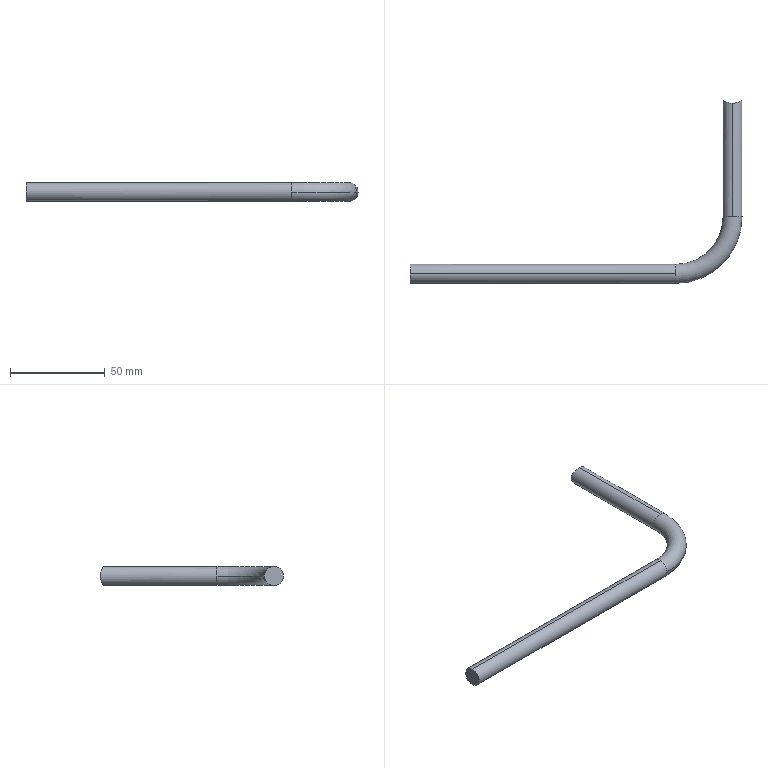Part | SolidWorks | features ICE 1, Sweep 1 | 1 solid | 8 faces | box 175 x 96.34 x 10 mm | volume 19434 mm3 | cylinder 5 | torus 2 | plane 1 | commonest cylinder face diameters 10 x4 20 x1
STEP:
#1=CARTESIAN_POINT('',(140.,0.,5.));
#2=VERTEX_POINT('',#1);
#3=CARTESIAN_POINT('',(140.,-5.,0.));
#4=VERTEX_POINT('',#3);
#5=CARTESIAN_POINT('',(140.,0.,0.));
#6=DIRECTION('',(1.,0.,0.));
#7=DIRECTION('',(0.,0.,-1.));
#8=AXIS2_PLACEMENT_3D('',#5,#6,#7);
#9=CIRCLE('',#8,5.);
#10=EDGE_CURVE('',#2,#4,#9,.T.);
#11=ORIENTED_EDGE('',*,*,#10,.T.);
#12=CARTESIAN_POINT('',(175.,30.,0.));
#13=VERTEX_POINT('',#12);
#14=CARTESIAN_POINT('',(140.,30.,0.));
#15=DIRECTION('',(0.,0.,1.));
#16=DIRECTION('',(1.,0.,0.));
#17=AXIS2_PLACEMENT_3D('',#14,#15,#16);
#18=CIRCLE('',#17,35.);
#19=EDGE_CURVE('',#4,#13,#18,.T.);
#20=ORIENTED_EDGE('',*,*,#19,.T.);
#21=CARTESIAN_POINT('',(170.,30.,5.));
#22=VERTEX_POINT('',#21);
#23=CARTESIAN_POINT('',(170.,30.,0.));
#24=DIRECTION('',(0.,1.,0.));
#25=DIRECTION('',(0.,0.,-1.));
#26=AXIS2_PLACEMENT_3D('',#23,#24,#25);
#27=CIRCLE('',#26,5.);
#28=EDGE_CURVE('',#22,#13,#27,.T.);
#29=ORIENTED_EDGE('',*,*,#28,.F.);
#30=CARTESIAN_POINT('',(165.,30.,0.));
#31=VERTEX_POINT('',#30);
#32=CARTESIAN_POINT('',(170.,30.,0.));
#33=DIRECTION('',(0.,1.,0.));
#34=DIRECTION('',(0.,0.,-1.));
#35=AXIS2_PLACEMENT_3D('',#32,#33,#34);
#36=CIRCLE('',#35,5.);
#37=EDGE_CURVE('',#31,#22,#36,.T.);
#38=ORIENTED_EDGE('',*,*,#37,.F.);
#39=CARTESIAN_POINT('',(140.,5.,0.));
#40=VERTEX_POINT('',#39);
#41=CARTESIAN_POINT('',(140.,30.,0.));
#42=DIRECTION('',(0.,0.,1.));
#43=DIRECTION('',(1.,0.,0.));
#44=AXIS2_PLACEMENT_3D('',#41,#42,#43);
#45=CIRCLE('',#44,25.);
#46=EDGE_CURVE('',#40,#31,#45,.T.);
#47=ORIENTED_EDGE('',*,*,#46,.F.);
#48=CARTESIAN_POINT('',(140.,0.,0.));
#49=DIRECTION('',(1.,0.,0.));
#50=DIRECTION('',(0.,0.,-1.));
#51=AXIS2_PLACEMENT_3D('',#48,#49,#50);
#52=CIRCLE('',#51,5.);
#53=EDGE_CURVE('',#40,#2,#52,.T.);
#54=ORIENTED_EDGE('',*,*,#53,.T.);
#55=EDGE_LOOP('',(#11,#20,#29,#38,#47,#54));
#56=FACE_OUTER_BOUND('',#55,.T.);
#57=CARTESIAN_POINT('',(140.,30.,0.));
#58=DIRECTION('',(0.,0.,1.));
#59=DIRECTION('',(1.,0.,0.));
#60=AXIS2_PLACEMENT_3D('',#57,#58,#59);
#61=TOROIDAL_SURFACE('',#60,30.,5.);
#62=ADVANCED_FACE('',(#56),#61,.T.);
#63=ORIENTED_EDGE('',*,*,#28,.T.);
#64=CARTESIAN_POINT('',(170.,30.,-5.));
#65=VERTEX_POINT('',#64);
#66=CARTESIAN_POINT('',(170.,30.,0.));
#67=DIRECTION('',(0.,1.,0.));
#68=DIRECTION('',(0.,0.,-1.));
#69=AXIS2_PLACEMENT_3D('',#66,#67,#68);
#70=CIRCLE('',#69,5.);
#71=EDGE_CURVE('',#13,#65,#70,.T.);
#72=ORIENTED_EDGE('',*,*,#71,.T.);
#73=CARTESIAN_POINT('',(170.,90.,-5.));
#74=VERTEX_POINT('',#73);
#75=CARTESIAN_POINT('',(170.,30.,-5.));
#76=DIRECTION('',(0.,1.,0.));
#77=VECTOR('',#76,1000.);
#78=LINE('',#75,#77);
#79=EDGE_CURVE('',#65,#74,#78,.T.);
#80=ORIENTED_EDGE('',*,*,#79,.T.);
#81=CARTESIAN_POINT('',(170.,90.,5.));
#82=VERTEX_POINT('',#81);
#83=CARTESIAN_POINT('',(170.,90.,5.));
#84=CARTESIAN_POINT('',(170.336,90.,5.));
#85=CARTESIAN_POINT('',(170.666,90.017,4.966));
#86=CARTESIAN_POINT('',(171.314,90.081,4.836));
#87=CARTESIAN_POINT('',(171.634,90.13,4.737));
#88=CARTESIAN_POINT('',(172.238,90.249,4.483));
#89=CARTESIAN_POINT('',(172.523,90.32,4.329));
#90=CARTESIAN_POINT('',(173.063,90.476,3.965));
#91=CARTESIAN_POINT('',(173.313,90.562,3.758));
#92=CARTESIAN_POINT('',(173.766,90.733,3.305));
#93=CARTESIAN_POINT('',(173.972,90.821,3.054));
#94=CARTESIAN_POINT('',(174.333,90.985,2.516));
#95=CARTESIAN_POINT('',(174.486,91.061,2.232));
#96=CARTESIAN_POINT('',(174.674,91.159,1.783));
#97=CARTESIAN_POINT('',(174.73,91.189,1.629));
#98=CARTESIAN_POINT('',(174.827,91.242,1.313));
#99=CARTESIAN_POINT('',(174.868,91.265,1.152));
#100=CARTESIAN_POINT('',(174.966,91.32,0.6658));
#101=CARTESIAN_POINT('',(175.,91.34,0.3376));
#102=CARTESIAN_POINT('',(175.,91.34,-0.1616));
#103=CARTESIAN_POINT('',(174.992,91.335,-0.3303));
#104=CARTESIAN_POINT('',(174.959,91.316,-0.6628));
#105=CARTESIAN_POINT('',(174.934,91.302,-0.8268));
#106=CARTESIAN_POINT('',(174.836,91.247,-1.312));
#107=CARTESIAN_POINT('',(174.738,91.193,-1.63));
#108=CARTESIAN_POINT('',(174.485,91.061,-2.235));
#109=CARTESIAN_POINT('',(174.331,90.984,-2.52));
#110=CARTESIAN_POINT('',(173.97,90.82,-3.057));
#111=CARTESIAN_POINT('',(173.763,90.732,-3.308));
#112=CARTESIAN_POINT('',(173.309,90.56,-3.762));
#113=CARTESIAN_POINT('',(173.061,90.476,-3.967));
#114=CARTESIAN_POINT('',(172.52,90.319,-4.331));
#115=CARTESIAN_POINT('',(172.233,90.248,-4.486));
#116=CARTESIAN_POINT('',(171.783,90.159,-4.674));
#117=CARTESIAN_POINT('',(171.629,90.132,-4.73));
#118=CARTESIAN_POINT('',(171.314,90.085,-4.827));
#119=CARTESIAN_POINT('',(171.152,90.065,-4.868));
#120=CARTESIAN_POINT('',(170.661,90.016,-4.967));
#121=CARTESIAN_POINT('',(170.332,90.,-5.));
#122=CARTESIAN_POINT('',(170.,90.,-5.));
#123=B_SPLINE_CURVE_WITH_KNOTS('',3,(#83,#84,#85,#86,#87,#88,#89,#90,#91,#92,#93,#94,#95,#96,#97,#98,#99,#100,#101,#102,#103,#104,#105,#106,#107,#108,#109,#110,#111,#112,#113,#114,#115,#116,#117,#118,#119,#120,#121,#122),.UNSPECIFIED.,.F.,.F.,(4,2,2,2,2,2,2,2,2,2,2,2,2,2,2,2,2,2,2,4),(0.,0.0009941,0.001988,0.002982,0.003976,0.00497,0.005964,0.006461,0.006958,0.007952,0.008449,0.008947,0.009941,0.01093,0.01193,0.01292,0.01392,0.01441,0.01491,0.0159),.UNSPECIFIED.);
#124=EDGE_CURVE('',#82,#74,#123,.T.);
#125=ORIENTED_EDGE('',*,*,#124,.F.);
#126=CARTESIAN_POINT('',(170.,30.,5.));
#127=DIRECTION('',(0.,1.,0.));
#128=VECTOR('',#127,1000.);
#129=LINE('',#126,#128);
#130=EDGE_CURVE('',#22,#82,#129,.T.);
#131=ORIENTED_EDGE('',*,*,#130,.F.);
#132=EDGE_LOOP('',(#63,#72,#80,#125,#131));
#133=FACE_OUTER_BOUND('',#132,.T.);
#134=CARTESIAN_POINT('',(170.,30.,0.));
#135=DIRECTION('',(0.,1.,0.));
#136=DIRECTION('',(0.,0.,1.));
#137=AXIS2_PLACEMENT_3D('',#134,#135,#136);
#138=CYLINDRICAL_SURFACE('',#137,5.);
#139=ADVANCED_FACE('',(#133),#138,.T.);
#140=CARTESIAN_POINT('',(0.,0.,-5.));
#141=VERTEX_POINT('',#140);
#142=CARTESIAN_POINT('',(0.,0.,5.));
#143=VERTEX_POINT('',#142);
#144=CARTESIAN_POINT('',(0.,0.,0.));
#145=DIRECTION('',(1.,0.,0.));
#146=DIRECTION('',(0.,0.,-1.));
#147=AXIS2_PLACEMENT_3D('',#144,#145,#146);
#148=CIRCLE('',#147,5.);
#149=EDGE_CURVE('',#141,#143,#148,.T.);
#150=ORIENTED_EDGE('',*,*,#149,.T.);
#151=CARTESIAN_POINT('',(0.,0.,5.));
#152=DIRECTION('',(1.,0.,0.));
#153=VECTOR('',#152,1000.);
#154=LINE('',#151,#153);
#155=EDGE_CURVE('',#143,#2,#154,.T.);
#156=ORIENTED_EDGE('',*,*,#155,.T.);
#157=ORIENTED_EDGE('',*,*,#53,.F.);
#158=CARTESIAN_POINT('',(140.,0.,-5.));
#159=VERTEX_POINT('',#158);
#160=CARTESIAN_POINT('',(140.,0.,0.));
#161=DIRECTION('',(1.,0.,0.));
#162=DIRECTION('',(0.,0.,-1.));
#163=AXIS2_PLACEMENT_3D('',#160,#161,#162);
#164=CIRCLE('',#163,5.);
#165=EDGE_CURVE('',#159,#40,#164,.T.);
#166=ORIENTED_EDGE('',*,*,#165,.F.);
#167=CARTESIAN_POINT('',(0.,0.,-5.));
#168=DIRECTION('',(1.,0.,0.));
#169=VECTOR('',#168,1000.);
#170=LINE('',#167,#169);
#171=EDGE_CURVE('',#141,#159,#170,.T.);
#172=ORIENTED_EDGE('',*,*,#171,.F.);
#173=EDGE_LOOP('',(#150,#156,#157,#166,#172));
#174=FACE_OUTER_BOUND('',#173,.T.);
#175=CARTESIAN_POINT('',(0.,0.,0.));
#176=DIRECTION('',(1.,0.,0.));
#177=DIRECTION('',(0.,0.,-1.));
#178=AXIS2_PLACEMENT_3D('',#175,#176,#177);
#179=CYLINDRICAL_SURFACE('',#178,5.);
#180=ADVANCED_FACE('',(#174),#179,.T.);
#181=ORIENTED_EDGE('',*,*,#79,.F.);
#182=CARTESIAN_POINT('',(170.,30.,0.));
#183=DIRECTION('',(0.,1.,0.));
#184=DIRECTION('',(0.,0.,-1.));
#185=AXIS2_PLACEMENT_3D('',#182,#183,#184);
#186=CIRCLE('',#185,5.);
#187=EDGE_CURVE('',#65,#31,#186,.T.);
#188=ORIENTED_EDGE('',*,*,#187,.T.);
#189=ORIENTED_EDGE('',*,*,#37,.T.);
#190=ORIENTED_EDGE('',*,*,#130,.T.);
#191=CARTESIAN_POINT('',(170.,90.,-5.));
#192=CARTESIAN_POINT('',(169.669,90.,-5.));
#193=CARTESIAN_POINT('',(169.331,90.017,-4.966));
#194=CARTESIAN_POINT('',(168.683,90.082,-4.835));
#195=CARTESIAN_POINT('',(168.369,90.129,-4.738));
#196=CARTESIAN_POINT('',(167.76,90.249,-4.482));
#197=CARTESIAN_POINT('',(167.474,90.32,-4.327));
#198=CARTESIAN_POINT('',(166.939,90.476,-3.966));
#199=CARTESIAN_POINT('',(166.686,90.562,-3.758));
#200=CARTESIAN_POINT('',(166.233,90.734,-3.303));
#201=CARTESIAN_POINT('',(166.029,90.82,-3.056));
#202=CARTESIAN_POINT('',(165.669,90.984,-2.52));
#203=CARTESIAN_POINT('',(165.513,91.062,-2.231));
#204=CARTESIAN_POINT('',(165.263,91.192,-1.633));
#205=CARTESIAN_POINT('',(165.166,91.246,-1.321));
#206=CARTESIAN_POINT('',(165.067,91.301,-0.8319));
#207=CARTESIAN_POINT('',(165.042,91.316,-0.666));
#208=CARTESIAN_POINT('',(165.009,91.335,-0.3359));
#209=CARTESIAN_POINT('',(164.992,91.344,-0.005573));
#210=CARTESIAN_POINT('',(165.008,91.335,0.3254));
#211=CARTESIAN_POINT('',(165.041,91.316,0.6568));
#212=CARTESIAN_POINT('',(165.065,91.302,0.8234));
#213=CARTESIAN_POINT('',(165.164,91.247,1.311));
#214=CARTESIAN_POINT('',(165.26,91.194,1.625));
#215=CARTESIAN_POINT('',(165.513,91.062,2.23));
#216=CARTESIAN_POINT('',(165.668,90.985,2.518));
#217=CARTESIAN_POINT('',(166.027,90.821,3.053));
#218=CARTESIAN_POINT('',(166.233,90.733,3.304));
#219=CARTESIAN_POINT('',(166.689,90.561,3.761));
#220=CARTESIAN_POINT('',(166.936,90.477,3.965));
#221=CARTESIAN_POINT('',(167.472,90.321,4.326));
#222=CARTESIAN_POINT('',(167.763,90.249,4.483));
#223=CARTESIAN_POINT('',(168.365,90.13,4.736));
#224=CARTESIAN_POINT('',(168.677,90.082,4.833));
#225=CARTESIAN_POINT('',(169.326,90.017,4.965));
#226=CARTESIAN_POINT('',(169.664,90.,5.));
#227=CARTESIAN_POINT('',(170.,90.,5.));
#228=B_SPLINE_CURVE_WITH_KNOTS('',3,(#191,#192,#193,#194,#195,#196,#197,#198,#199,#200,#201,#202,#203,#204,#205,#206,#207,#208,#209,#210,#211,#212,#213,#214,#215,#216,#217,#218,#219,#220,#221,#222,#223,#224,#225,#226,#227),.UNSPECIFIED.,.F.,.F.,(4,2,2,2,2,2,2,2,2,1,2,2,2,2,2,2,2,2,4),(0.0159,0.0169,0.01789,0.01888,0.01987,0.02087,0.02186,0.02285,0.02335,0.02384,0.02434,0.02484,0.02583,0.02682,0.02781,0.02881,0.0298,0.03079,0.03178),.UNSPECIFIED.);
#229=EDGE_CURVE('',#74,#82,#228,.T.);
#230=ORIENTED_EDGE('',*,*,#229,.F.);
#231=EDGE_LOOP('',(#181,#188,#189,#190,#230));
#232=FACE_OUTER_BOUND('',#231,.T.);
#233=CARTESIAN_POINT('',(170.,30.,0.));
#234=DIRECTION('',(0.,1.,0.));
#235=DIRECTION('',(0.,0.,1.));
#236=AXIS2_PLACEMENT_3D('',#233,#234,#235);
#237=CYLINDRICAL_SURFACE('',#236,5.);
#238=ADVANCED_FACE('',(#232),#237,.T.);
#239=ORIENTED_EDGE('',*,*,#19,.F.);
#240=CARTESIAN_POINT('',(140.,0.,0.));
#241=DIRECTION('',(1.,0.,0.));
#242=DIRECTION('',(0.,0.,-1.));
#243=AXIS2_PLACEMENT_3D('',#240,#241,#242);
#244=CIRCLE('',#243,5.);
#245=EDGE_CURVE('',#4,#159,#244,.T.);
#246=ORIENTED_EDGE('',*,*,#245,.T.);
#247=ORIENTED_EDGE('',*,*,#165,.T.);
#248=ORIENTED_EDGE('',*,*,#46,.T.);
#249=ORIENTED_EDGE('',*,*,#187,.F.);
#250=ORIENTED_EDGE('',*,*,#71,.F.);
#251=EDGE_LOOP('',(#239,#246,#247,#248,#249,#250));
#252=FACE_OUTER_BOUND('',#251,.T.);
#253=CARTESIAN_POINT('',(140.,30.,0.));
#254=DIRECTION('',(0.,0.,1.));
#255=DIRECTION('',(1.,0.,0.));
#256=AXIS2_PLACEMENT_3D('',#253,#254,#255);
#257=TOROIDAL_SURFACE('',#256,30.,5.);
#258=ADVANCED_FACE('',(#252),#257,.T.);
#259=ORIENTED_EDGE('',*,*,#155,.F.);
#260=CARTESIAN_POINT('',(0.,0.,0.));
#261=DIRECTION('',(1.,0.,0.));
#262=DIRECTION('',(0.,0.,-1.));
#263=AXIS2_PLACEMENT_3D('',#260,#261,#262);
#264=CIRCLE('',#263,5.);
#265=EDGE_CURVE('',#143,#141,#264,.T.);
#266=ORIENTED_EDGE('',*,*,#265,.T.);
#267=ORIENTED_EDGE('',*,*,#171,.T.);
#268=ORIENTED_EDGE('',*,*,#245,.F.);
#269=ORIENTED_EDGE('',*,*,#10,.F.);
#270=EDGE_LOOP('',(#259,#266,#267,#268,#269));
#271=FACE_OUTER_BOUND('',#270,.T.);
#272=CARTESIAN_POINT('',(0.,0.,0.));
#273=DIRECTION('',(1.,0.,0.));
#274=DIRECTION('',(0.,0.,-1.));
#275=AXIS2_PLACEMENT_3D('',#272,#273,#274);
#276=CYLINDRICAL_SURFACE('',#275,5.);
#277=ADVANCED_FACE('',(#271),#276,.T.);
#278=ORIENTED_EDGE('',*,*,#149,.F.);
#279=ORIENTED_EDGE('',*,*,#265,.F.);
#280=EDGE_LOOP('',(#278,#279));
#281=FACE_OUTER_BOUND('',#280,.T.);
#282=CARTESIAN_POINT('',(0.,0.,0.));
#283=DIRECTION('',(1.,0.,0.));
#284=DIRECTION('',(0.,0.,-1.));
#285=AXIS2_PLACEMENT_3D('',#282,#283,#284);
#286=PLANE('',#285);
#287=ADVANCED_FACE('',(#281),#286,.F.);
#288=ORIENTED_EDGE('',*,*,#124,.T.);
#289=ORIENTED_EDGE('',*,*,#229,.T.);
#290=EDGE_LOOP('',(#288,#289));
#291=FACE_OUTER_BOUND('',#290,.T.);
#292=CARTESIAN_POINT('',(170.,100.,-5.));
#293=DIRECTION('',(0.,0.,1.));
#294=DIRECTION('',(1.,0.,0.));
#295=AXIS2_PLACEMENT_3D('',#292,#293,#294);
#296=CYLINDRICAL_SURFACE('',#295,10.);
#297=ADVANCED_FACE('',(#291),#296,.F.);
#298=CLOSED_SHELL('',(#62,#139,#180,#238,#258,#277,#287,#297));
#299=MANIFOLD_SOLID_BREP('',#298);
#300=CARTESIAN_POINT('',(0.,0.,0.));
#301=DIRECTION('',(0.,0.,1.));
#302=DIRECTION('',(1.,0.,0.));
#303=AXIS2_PLACEMENT_3D('',#300,#301,#302);
#304=(LENGTH_UNIT()NAMED_UNIT(*)SI_UNIT(.MILLI.,.METRE.));
#305=UNCERTAINTY_MEASURE_WITH_UNIT(LENGTH_MEASURE(0.00001),#304,'','');
#306=(NAMED_UNIT(*)PLANE_ANGLE_UNIT()SI_UNIT($,.RADIAN.));
#307=(NAMED_UNIT(*)SI_UNIT($,.STERADIAN.)SOLID_ANGLE_UNIT());
#308=(GEOMETRIC_REPRESENTATION_CONTEXT(3)GLOBAL_UNCERTAINTY_ASSIGNED_CONTEXT((#305))GLOBAL_UNIT_ASSIGNED_CONTEXT((#304,#306,#307))REPRESENTATION_CONTEXT('',''));
#309=ADVANCED_BREP_SHAPE_REPRESENTATION('',(#299,#303),#308);